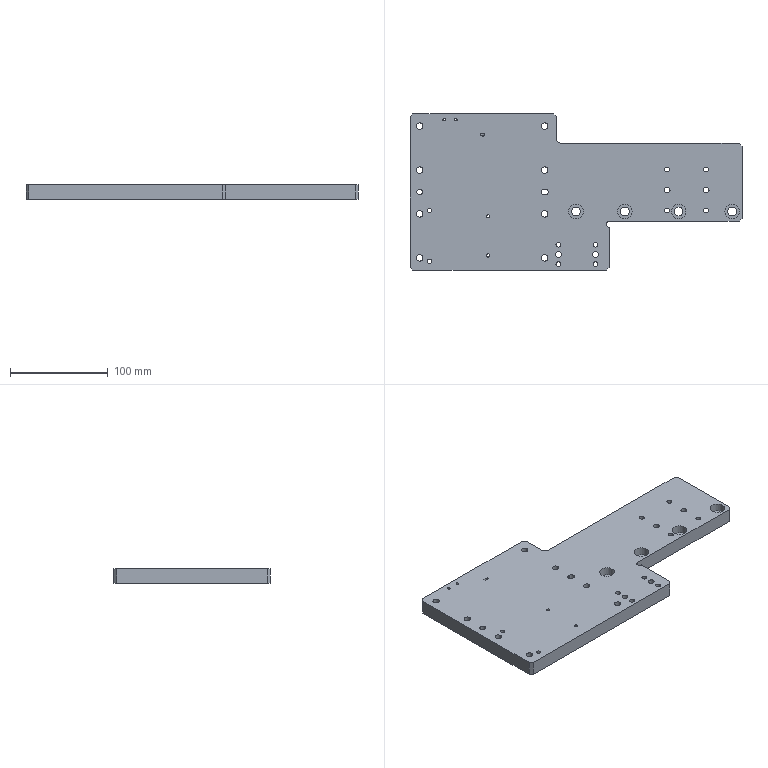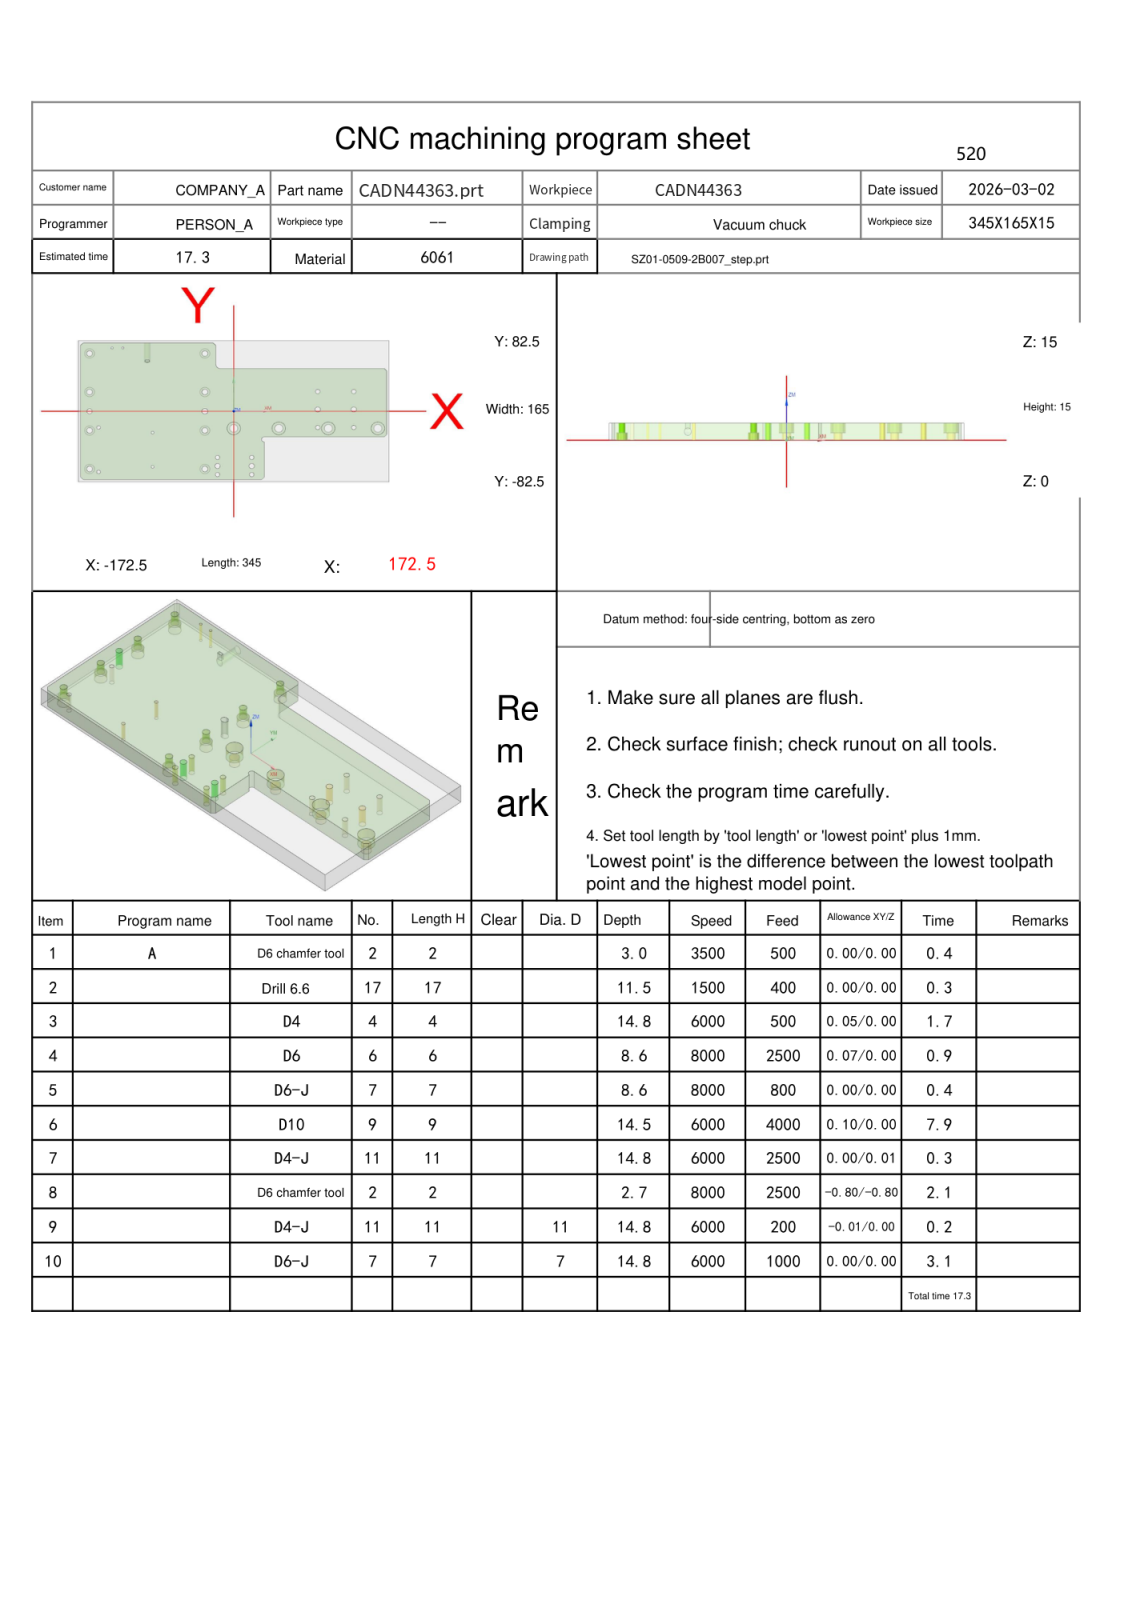NC program | NX | posted by the shop | part box 340 x 160 x 15 mm
Lines 978 to 1830 of 3961:
N6 T09 M06
(D10  D=10. R=0. H=09 ce=0.10 di=0.00)
G00 G90 G54 X-68. Y-85.1 M03 S6000
G43 H09 Z65.
M08
Z15.5
G01 X-167. Z15.451 F4000.
G02 X-170.606 Y-83.606 Z15.449 I0.0 J5.1
G01 X-173.606 Y-80.606 Z15.447
G02 X-175.1 Y-77. Z15.445 I3.606 J3.606
G01 Y77. Z15.37
G02 X-173.606 Y80.606 Z15.368 I5.1 J0.0
G01 X-170.606 Y83.606 Z15.366
G02 X-167. Y85.1 Z15.364 I3.606 J-3.606
G01 X-23. Z15.293
G02 X-19.394 Y83.606 Z15.291 I0.0 J-5.1
G01 X-16.394 Y80.606 Z15.289
G02 X-14.9 Y77. Z15.287 I-3.606 J-3.606
G01 Y55.1 Z15.276
X167. Z15.187
G02 X170.606 Y53.606 Z15.185 I0.0 J-5.1
G01 X173.606 Y50.606 Z15.183
G02 X175.1 Y47. Z15.181 I-3.606 J-3.606
G01 Y-27. Z15.144
G02 X173.606 Y-30.606 Z15.142 I-5.1 J0.0
G01 X170.606 Y-33.606 Z15.14
G02 X167. Y-35.1 Z15.138 I-3.606 J3.606
G01 X39.02 Z15.075
G02 X39.1 Y-36. Z15.075 I-5.02 J-.9
G01 Y-77. Z15.055
G02 X37.606 Y-80.606 Z15.053 I-5.1 J0.0
G01 X34.606 Y-83.606 Z15.051
G02 X31. Y-85.1 Z15.049 I-3.606 J3.606
G01 X-167. Z14.951
G02 X-170.606 Y-83.606 Z14.949 I0.0 J5.1
G01 X-173.606 Y-80.606 Z14.947
G02 X-175.1 Y-77. Z14.945 I3.606 J3.606
G01 Y77. Z14.87
G02 X-173.606 Y80.606 Z14.868 I5.1 J0.0
G01 X-170.606 Y83.606 Z14.866
G02 X-167. Y85.1 Z14.864 I3.606 J-3.606
G01 X-23. Z14.793
G02 X-19.394 Y83.606 Z14.791 I0.0 J-5.1
G01 X-16.394 Y80.606 Z14.789
G02 X-14.9 Y77. Z14.787 I-3.606 J-3.606
G01 Y55.1 Z14.776
X167. Z14.687
G02 X170.606 Y53.606 Z14.685 I0.0 J-5.1
G01 X173.606 Y50.606 Z14.683
G02 X175.1 Y47. Z14.681 I-3.606 J-3.606
G01 Y-27. Z14.644
G02 X173.606 Y-30.606 Z14.642 I-5.1 J0.0
G01 X170.606 Y-33.606 Z14.64
G02 X167. Y-35.1 Z14.638 I-3.606 J3.606
G01 X39.02 Z14.575
G02 X39.1 Y-36. Z14.575 I-5.02 J-.9
G01 Y-77. Z14.555
G02 X37.606 Y-80.606 Z14.553 I-5.1 J0.0
G01 X34.606 Y-83.606 Z14.551
G02 X31. Y-85.1 Z14.549 I-3.606 J3.606
G01 X-167. Z14.451
G02 X-170.606 Y-83.606 Z14.449 I0.0 J5.1
G01 X-173.606 Y-80.606 Z14.447
G02 X-175.1 Y-77. Z14.445 I3.606 J3.606
G01 Y77. Z14.37
G02 X-173.606 Y80.606 Z14.368 I5.1 J0.0
G01 X-170.606 Y83.606 Z14.366
G02 X-167. Y85.1 Z14.364 I3.606 J-3.606
G01 X-23. Z14.293
G02 X-19.394 Y83.606 Z14.291 I0.0 J-5.1
G01 X-16.394 Y80.606 Z14.289
G02 X-14.9 Y77. Z14.287 I-3.606 J-3.606
G01 Y55.1 Z14.276
X167. Z14.187
G02 X170.606 Y53.606 Z14.185 I0.0 J-5.1
G01 X173.606 Y50.606 Z14.183
G02 X175.1 Y47. Z14.181 I-3.606 J-3.606
G01 Y-27. Z14.144
G02 X173.606 Y-30.606 Z14.142 I-5.1 J0.0
G01 X170.606 Y-33.606 Z14.14
G02 X167. Y-35.1 Z14.138 I-3.606 J3.606
G01 X39.02 Z14.075
G02 X39.1 Y-36. Z14.075 I-5.02 J-.9
G01 Y-77. Z14.055
G02 X37.606 Y-80.606 Z14.053 I-5.1 J0.0
G01 X34.606 Y-83.606 Z14.051
G02 X31. Y-85.1 Z14.049 I-3.606 J3.606
G01 X-167. Z13.951
G02 X-170.606 Y-83.606 Z13.949 I0.0 J5.1
G01 X-173.606 Y-80.606 Z13.947
G02 X-175.1 Y-77. Z13.945 I3.606 J3.606
G01 Y77. Z13.87
G02 X-173.606 Y80.606 Z13.868 I5.1 J0.0
G01 X-170.606 Y83.606 Z13.866
G02 X-167. Y85.1 Z13.864 I3.606 J-3.606
G01 X-23. Z13.793
G02 X-19.394 Y83.606 Z13.791 I0.0 J-5.1
G01 X-16.394 Y80.606 Z13.789
G02 X-14.9 Y77. Z13.787 I-3.606 J-3.606
G01 Y55.1 Z13.776
X167. Z13.687
G02 X170.606 Y53.606 Z13.685 I0.0 J-5.1
G01 X173.606 Y50.606 Z13.683
G02 X175.1 Y47. Z13.681 I-3.606 J-3.606
G01 Y-27. Z13.644
G02 X173.606 Y-30.606 Z13.642 I-5.1 J0.0
G01 X170.606 Y-33.606 Z13.64
G02 X167. Y-35.1 Z13.638 I-3.606 J3.606
G01 X39.02 Z13.575
G02 X39.1 Y-36. Z13.575 I-5.02 J-.9
G01 Y-77. Z13.555
G02 X37.606 Y-80.606 Z13.553 I-5.1 J0.0
G01 X34.606 Y-83.606 Z13.551
G02 X31. Y-85.1 Z13.549 I-3.606 J3.606
G01 X-167. Z13.451
G02 X-170.606 Y-83.606 Z13.449 I0.0 J5.1
G01 X-173.606 Y-80.606 Z13.447
G02 X-175.1 Y-77. Z13.445 I3.606 J3.606
G01 Y77. Z13.37
G02 X-173.606 Y80.606 Z13.368 I5.1 J0.0
G01 X-170.606 Y83.606 Z13.366
G02 X-167. Y85.1 Z13.364 I3.606 J-3.606
G01 X-23. Z13.293
G02 X-19.394 Y83.606 Z13.291 I0.0 J-5.1
G01 X-16.394 Y80.606 Z13.289
G02 X-14.9 Y77. Z13.287 I-3.606 J-3.606
G01 Y55.1 Z13.276
X167. Z13.187
G02 X170.606 Y53.606 Z13.185 I0.0 J-5.1
G01 X173.606 Y50.606 Z13.183
G02 X175.1 Y47. Z13.181 I-3.606 J-3.606
G01 Y-27. Z13.144
G02 X173.606 Y-30.606 Z13.142 I-5.1 J0.0
G01 X170.606 Y-33.606 Z13.14
G02 X167. Y-35.1 Z13.138 I-3.606 J3.606
G01 X39.02 Z13.075
G02 X39.1 Y-36. Z13.075 I-5.02 J-.9
G01 Y-77. Z13.055
G02 X37.606 Y-80.606 Z13.053 I-5.1 J0.0
G01 X34.606 Y-83.606 Z13.051
G02 X31. Y-85.1 Z13.049 I-3.606 J3.606
G01 X-167. Z12.951
G02 X-170.606 Y-83.606 Z12.949 I0.0 J5.1
G01 X-173.606 Y-80.606 Z12.947
G02 X-175.1 Y-77. Z12.945 I3.606 J3.606
G01 Y77. Z12.87
G02 X-173.606 Y80.606 Z12.868 I5.1 J0.0
G01 X-170.606 Y83.606 Z12.866
G02 X-167. Y85.1 Z12.864 I3.606 J-3.606
G01 X-23. Z12.793
G02 X-19.394 Y83.606 Z12.791 I0.0 J-5.1
G01 X-16.394 Y80.606 Z12.789
G02 X-14.9 Y77. Z12.787 I-3.606 J-3.606
G01 Y55.1 Z12.776
X167. Z12.687
G02 X170.606 Y53.606 Z12.685 I0.0 J-5.1
G01 X173.606 Y50.606 Z12.683
G02 X175.1 Y47. Z12.681 I-3.606 J-3.606
G01 Y-27. Z12.644
G02 X173.606 Y-30.606 Z12.642 I-5.1 J0.0
G01 X170.606 Y-33.606 Z12.64
G02 X167. Y-35.1 Z12.638 I-3.606 J3.606
G01 X39.02 Z12.575
G02 X39.1 Y-36. Z12.575 I-5.02 J-.9
G01 Y-77. Z12.555
G02 X37.606 Y-80.606 Z12.553 I-5.1 J0.0
G01 X34.606 Y-83.606 Z12.551
G02 X31. Y-85.1 Z12.549 I-3.606 J3.606
G01 X-167. Z12.451
G02 X-170.606 Y-83.606 Z12.449 I0.0 J5.1
G01 X-173.606 Y-80.606 Z12.447
G02 X-175.1 Y-77. Z12.445 I3.606 J3.606
G01 Y77. Z12.37
G02 X-173.606 Y80.606 Z12.368 I5.1 J0.0
G01 X-170.606 Y83.606 Z12.366
G02 X-167. Y85.1 Z12.364 I3.606 J-3.606
G01 X-23. Z12.293
G02 X-19.394 Y83.606 Z12.291 I0.0 J-5.1
G01 X-16.394 Y80.606 Z12.289
G02 X-14.9 Y77. Z12.287 I-3.606 J-3.606
G01 Y55.1 Z12.276
X167. Z12.187
G02 X170.606 Y53.606 Z12.185 I0.0 J-5.1
G01 X173.606 Y50.606 Z12.183
G02 X175.1 Y47. Z12.181 I-3.606 J-3.606
G01 Y-27. Z12.144
G02 X173.606 Y-30.606 Z12.142 I-5.1 J0.0
G01 X170.606 Y-33.606 Z12.14
G02 X167. Y-35.1 Z12.138 I-3.606 J3.606
G01 X39.02 Z12.075
G02 X39.1 Y-36. Z12.075 I-5.02 J-.9
G01 Y-77. Z12.055
G02 X37.606 Y-80.606 Z12.053 I-5.1 J0.0
G01 X34.606 Y-83.606 Z12.051
G02 X31. Y-85.1 Z12.049 I-3.606 J3.606
G01 X-167. Z11.951
G02 X-170.606 Y-83.606 Z11.949 I0.0 J5.1
G01 X-173.606 Y-80.606 Z11.947
G02 X-175.1 Y-77. Z11.945 I3.606 J3.606
G01 Y77. Z11.87
G02 X-173.606 Y80.606 Z11.868 I5.1 J0.0
G01 X-170.606 Y83.606 Z11.866
G02 X-167. Y85.1 Z11.864 I3.606 J-3.606
G01 X-23. Z11.793
G02 X-19.394 Y83.606 Z11.791 I0.0 J-5.1
G01 X-16.394 Y80.606 Z11.789
G02 X-14.9 Y77. Z11.787 I-3.606 J-3.606
G01 Y55.1 Z11.776
X167. Z11.687
G02 X170.606 Y53.606 Z11.685 I0.0 J-5.1
G01 X173.606 Y50.606 Z11.683
G02 X175.1 Y47. Z11.681 I-3.606 J-3.606
G01 Y-27. Z11.644
G02 X173.606 Y-30.606 Z11.642 I-5.1 J0.0
G01 X170.606 Y-33.606 Z11.64
G02 X167. Y-35.1 Z11.638 I-3.606 J3.606
G01 X39.02 Z11.575
G02 X39.1 Y-36. Z11.575 I-5.02 J-.9
G01 Y-77. Z11.555
G02 X37.606 Y-80.606 Z11.553 I-5.1 J0.0
G01 X34.606 Y-83.606 Z11.551
G02 X31. Y-85.1 Z11.549 I-3.606 J3.606
G01 X-167. Z11.451
G02 X-170.606 Y-83.606 Z11.449 I0.0 J5.1
G01 X-173.606 Y-80.606 Z11.447
G02 X-175.1 Y-77. Z11.445 I3.606 J3.606
G01 Y77. Z11.37
G02 X-173.606 Y80.606 Z11.368 I5.1 J0.0
G01 X-170.606 Y83.606 Z11.366
G02 X-167. Y85.1 Z11.364 I3.606 J-3.606
G01 X-23. Z11.293
G02 X-19.394 Y83.606 Z11.291 I0.0 J-5.1
G01 X-16.394 Y80.606 Z11.289
G02 X-14.9 Y77. Z11.287 I-3.606 J-3.606
G01 Y55.1 Z11.276
X167. Z11.187
G02 X170.606 Y53.606 Z11.185 I0.0 J-5.1
G01 X173.606 Y50.606 Z11.183
G02 X175.1 Y47. Z11.181 I-3.606 J-3.606
G01 Y-27. Z11.144
G02 X173.606 Y-30.606 Z11.142 I-5.1 J0.0
G01 X170.606 Y-33.606 Z11.14
G02 X167. Y-35.1 Z11.138 I-3.606 J3.606
G01 X39.02 Z11.075
G02 X39.1 Y-36. Z11.075 I-5.02 J-.9
G01 Y-77. Z11.055
G02 X37.606 Y-80.606 Z11.053 I-5.1 J0.0
G01 X34.606 Y-83.606 Z11.051
G02 X31. Y-85.1 Z11.049 I-3.606 J3.606
G01 X-167. Z10.951
G02 X-170.606 Y-83.606 Z10.949 I0.0 J5.1
G01 X-173.606 Y-80.606 Z10.947
G02 X-175.1 Y-77. Z10.945 I3.606 J3.606
G01 Y77. Z10.87
G02 X-173.606 Y80.606 Z10.868 I5.1 J0.0
G01 X-170.606 Y83.606 Z10.866
G02 X-167. Y85.1 Z10.864 I3.606 J-3.606
G01 X-23. Z10.793
G02 X-19.394 Y83.606 Z10.791 I0.0 J-5.1
G01 X-16.394 Y80.606 Z10.789
G02 X-14.9 Y77. Z10.787 I-3.606 J-3.606
G01 Y55.1 Z10.776
X167. Z10.687
G02 X170.606 Y53.606 Z10.685 I0.0 J-5.1
G01 X173.606 Y50.606 Z10.683
G02 X175.1 Y47. Z10.681 I-3.606 J-3.606
G01 Y-27. Z10.644
G02 X173.606 Y-30.606 Z10.642 I-5.1 J0.0
G01 X170.606 Y-33.606 Z10.64
G02 X167. Y-35.1 Z10.638 I-3.606 J3.606
G01 X39.02 Z10.575
G02 X39.1 Y-36. Z10.575 I-5.02 J-.9
G01 Y-77. Z10.555
G02 X37.606 Y-80.606 Z10.553 I-5.1 J0.0
G01 X34.606 Y-83.606 Z10.551
G02 X31. Y-85.1 Z10.549 I-3.606 J3.606
G01 X-167. Z10.451
G02 X-170.606 Y-83.606 Z10.449 I0.0 J5.1
G01 X-173.606 Y-80.606 Z10.447
G02 X-175.1 Y-77. Z10.445 I3.606 J3.606
G01 Y77. Z10.37
G02 X-173.606 Y80.606 Z10.368 I5.1 J0.0
G01 X-170.606 Y83.606 Z10.366
G02 X-167. Y85.1 Z10.364 I3.606 J-3.606
G01 X-23. Z10.293
G02 X-19.394 Y83.606 Z10.291 I0.0 J-5.1
G01 X-16.394 Y80.606 Z10.289
G02 X-14.9 Y77. Z10.287 I-3.606 J-3.606
G01 Y55.1 Z10.276
X167. Z10.187
G02 X170.606 Y53.606 Z10.185 I0.0 J-5.1
G01 X173.606 Y50.606 Z10.183
G02 X175.1 Y47. Z10.181 I-3.606 J-3.606
G01 Y-27. Z10.144
G02 X173.606 Y-30.606 Z10.142 I-5.1 J0.0
G01 X170.606 Y-33.606 Z10.14
G02 X167. Y-35.1 Z10.138 I-3.606 J3.606
G01 X39.02 Z10.075
G02 X39.1 Y-36. Z10.075 I-5.02 J-.9
G01 Y-77. Z10.055
G02 X37.606 Y-80.606 Z10.053 I-5.1 J0.0
G01 X34.606 Y-83.606 Z10.051
G02 X31. Y-85.1 Z10.049 I-3.606 J3.606
G01 X-167. Z9.951
G02 X-170.606 Y-83.606 Z9.949 I0.0 J5.1
G01 X-173.606 Y-80.606 Z9.947
G02 X-175.1 Y-77. Z9.945 I3.606 J3.606
G01 Y77. Z9.87
G02 X-173.606 Y80.606 Z9.868 I5.1 J0.0
G01 X-170.606 Y83.606 Z9.866
G02 X-167. Y85.1 Z9.864 I3.606 J-3.606
G01 X-23. Z9.793
G02 X-19.394 Y83.606 Z9.791 I0.0 J-5.1
G01 X-16.394 Y80.606 Z9.789
G02 X-14.9 Y77. Z9.787 I-3.606 J-3.606
G01 Y55.1 Z9.776
X167. Z9.687
G02 X170.606 Y53.606 Z9.685 I0.0 J-5.1
G01 X173.606 Y50.606 Z9.683
G02 X175.1 Y47. Z9.681 I-3.606 J-3.606
G01 Y-27. Z9.644
G02 X173.606 Y-30.606 Z9.642 I-5.1 J0.0
G01 X170.606 Y-33.606 Z9.64
G02 X167. Y-35.1 Z9.638 I-3.606 J3.606
G01 X39.02 Z9.575
G02 X39.1 Y-36. Z9.575 I-5.02 J-.9
G01 Y-77. Z9.555
G02 X37.606 Y-80.606 Z9.553 I-5.1 J0.0
G01 X34.606 Y-83.606 Z9.551
G02 X31. Y-85.1 Z9.549 I-3.606 J3.606
G01 X-167. Z9.451
G02 X-170.606 Y-83.606 Z9.449 I0.0 J5.1
G01 X-173.606 Y-80.606 Z9.447
G02 X-175.1 Y-77. Z9.445 I3.606 J3.606
G01 Y77. Z9.37
G02 X-173.606 Y80.606 Z9.368 I5.1 J0.0
G01 X-170.606 Y83.606 Z9.366
G02 X-167. Y85.1 Z9.364 I3.606 J-3.606
G01 X-23. Z9.293
G02 X-19.394 Y83.606 Z9.291 I0.0 J-5.1
G01 X-16.394 Y80.606 Z9.289
G02 X-14.9 Y77. Z9.287 I-3.606 J-3.606
G01 Y55.1 Z9.276
X167. Z9.187
G02 X170.606 Y53.606 Z9.185 I0.0 J-5.1
G01 X173.606 Y50.606 Z9.183
G02 X175.1 Y47. Z9.181 I-3.606 J-3.606
G01 Y-27. Z9.144
G02 X173.606 Y-30.606 Z9.142 I-5.1 J0.0
G01 X170.606 Y-33.606 Z9.14
G02 X167. Y-35.1 Z9.138 I-3.606 J3.606
G01 X39.02 Z9.075
G02 X39.1 Y-36. Z9.075 I-5.02 J-.9
G01 Y-77. Z9.055
G02 X37.606 Y-80.606 Z9.053 I-5.1 J0.0
G01 X34.606 Y-83.606 Z9.051
G02 X31. Y-85.1 Z9.049 I-3.606 J3.606
G01 X-167. Z8.951
G02 X-170.606 Y-83.606 Z8.949 I0.0 J5.1
G01 X-173.606 Y-80.606 Z8.947
G02 X-175.1 Y-77. Z8.945 I3.606 J3.606
G01 Y77. Z8.87
G02 X-173.606 Y80.606 Z8.868 I5.1 J0.0
G01 X-170.606 Y83.606 Z8.866
G02 X-167. Y85.1 Z8.864 I3.606 J-3.606
G01 X-23. Z8.793
G02 X-19.394 Y83.606 Z8.791 I0.0 J-5.1
G01 X-16.394 Y80.606 Z8.789
G02 X-14.9 Y77. Z8.787 I-3.606 J-3.606
G01 Y55.1 Z8.776
X167. Z8.687
G02 X170.606 Y53.606 Z8.685 I0.0 J-5.1
G01 X173.606 Y50.606 Z8.683
G02 X175.1 Y47. Z8.681 I-3.606 J-3.606
G01 Y-27. Z8.644
G02 X173.606 Y-30.606 Z8.642 I-5.1 J0.0
G01 X170.606 Y-33.606 Z8.64
G02 X167. Y-35.1 Z8.638 I-3.606 J3.606
G01 X39.02 Z8.575
G02 X39.1 Y-36. Z8.575 I-5.02 J-.9
G01 Y-77. Z8.555
G02 X37.606 Y-80.606 Z8.553 I-5.1 J0.0
G01 X34.606 Y-83.606 Z8.551
G02 X31. Y-85.1 Z8.549 I-3.606 J3.606
G01 X-167. Z8.451
G02 X-170.606 Y-83.606 Z8.449 I0.0 J5.1
G01 X-173.606 Y-80.606 Z8.447
G02 X-175.1 Y-77. Z8.445 I3.606 J3.606
G01 Y77. Z8.37
G02 X-173.606 Y80.606 Z8.368 I5.1 J0.0
G01 X-170.606 Y83.606 Z8.366
G02 X-167. Y85.1 Z8.364 I3.606 J-3.606
G01 X-23. Z8.293
G02 X-19.394 Y83.606 Z8.291 I0.0 J-5.1
G01 X-16.394 Y80.606 Z8.289
G02 X-14.9 Y77. Z8.287 I-3.606 J-3.606
G01 Y55.1 Z8.276
X167. Z8.187
G02 X170.606 Y53.606 Z8.185 I0.0 J-5.1
G01 X173.606 Y50.606 Z8.183
G02 X175.1 Y47. Z8.181 I-3.606 J-3.606
G01 Y-27. Z8.144
G02 X173.606 Y-30.606 Z8.142 I-5.1 J0.0
G01 X170.606 Y-33.606 Z8.14
G02 X167. Y-35.1 Z8.138 I-3.606 J3.606
G01 X39.02 Z8.075
G02 X39.1 Y-36. Z8.075 I-5.02 J-.9
G01 Y-77. Z8.055
G02 X37.606 Y-80.606 Z8.053 I-5.1 J0.0
G01 X34.606 Y-83.606 Z8.051
G02 X31. Y-85.1 Z8.049 I-3.606 J3.606
G01 X-167. Z7.951
G02 X-170.606 Y-83.606 Z7.949 I0.0 J5.1
G01 X-173.606 Y-80.606 Z7.947
G02 X-175.1 Y-77. Z7.945 I3.606 J3.606
G01 Y77. Z7.87
G02 X-173.606 Y80.606 Z7.868 I5.1 J0.0
G01 X-170.606 Y83.606 Z7.866
G02 X-167. Y85.1 Z7.864 I3.606 J-3.606
G01 X-23. Z7.793
G02 X-19.394 Y83.606 Z7.791 I0.0 J-5.1
G01 X-16.394 Y80.606 Z7.789
G02 X-14.9 Y77. Z7.787 I-3.606 J-3.606
G01 Y55.1 Z7.776
X167. Z7.687
G02 X170.606 Y53.606 Z7.685 I0.0 J-5.1
G01 X173.606 Y50.606 Z7.683
G02 X175.1 Y47. Z7.681 I-3.606 J-3.606
G01 Y-27. Z7.644
G02 X173.606 Y-30.606 Z7.642 I-5.1 J0.0
G01 X170.606 Y-33.606 Z7.64
G02 X167. Y-35.1 Z7.638 I-3.606 J3.606
G01 X39.02 Z7.575
G02 X39.1 Y-36. Z7.575 I-5.02 J-.9
G01 Y-77. Z7.555
G02 X37.606 Y-80.606 Z7.553 I-5.1 J0.0
G01 X34.606 Y-83.606 Z7.551
G02 X31. Y-85.1 Z7.549 I-3.606 J3.606
G01 X-167. Z7.451
G02 X-170.606 Y-83.606 Z7.449 I0.0 J5.1
G01 X-173.606 Y-80.606 Z7.447
G02 X-175.1 Y-77. Z7.445 I3.606 J3.606
G01 Y77. Z7.37
G02 X-173.606 Y80.606 Z7.368 I5.1 J0.0
G01 X-170.606 Y83.606 Z7.366
G02 X-167. Y85.1 Z7.364 I3.606 J-3.606
G01 X-23. Z7.293
G02 X-19.394 Y83.606 Z7.291 I0.0 J-5.1
G01 X-16.394 Y80.606 Z7.289
G02 X-14.9 Y77. Z7.287 I-3.606 J-3.606
G01 Y55.1 Z7.276
X167. Z7.187
G02 X170.606 Y53.606 Z7.185 I0.0 J-5.1
G01 X173.606 Y50.606 Z7.183
G02 X175.1 Y47. Z7.181 I-3.606 J-3.606
G01 Y-27. Z7.144
G02 X173.606 Y-30.606 Z7.142 I-5.1 J0.0
G01 X170.606 Y-33.606 Z7.14
G02 X167. Y-35.1 Z7.138 I-3.606 J3.606
G01 X39.02 Z7.075
G02 X39.1 Y-36. Z7.075 I-5.02 J-.9
G01 Y-77. Z7.055
G02 X37.606 Y-80.606 Z7.053 I-5.1 J0.0
G01 X34.606 Y-83.606 Z7.051
G02 X31. Y-85.1 Z7.049 I-3.606 J3.606
G01 X-167. Z6.951
G02 X-170.606 Y-83.606 Z6.949 I0.0 J5.1
G01 X-173.606 Y-80.606 Z6.947
G02 X-175.1 Y-77. Z6.945 I3.606 J3.606
G01 Y77. Z6.87
G02 X-173.606 Y80.606 Z6.868 I5.1 J0.0
G01 X-170.606 Y83.606 Z6.866
G02 X-167. Y85.1 Z6.864 I3.606 J-3.606
G01 X-23. Z6.793
G02 X-19.394 Y83.606 Z6.791 I0.0 J-5.1
G01 X-16.394 Y80.606 Z6.789
G02 X-14.9 Y77. Z6.787 I-3.606 J-3.606
G01 Y55.1 Z6.776
X167. Z6.687
G02 X170.606 Y53.606 Z6.685 I0.0 J-5.1
G01 X173.606 Y50.606 Z6.683
G02 X175.1 Y47. Z6.681 I-3.606 J-3.606
G01 Y-27. Z6.644
G02 X173.606 Y-30.606 Z6.642 I-5.1 J0.0
G01 X170.606 Y-33.606 Z6.64
G02 X167. Y-35.1 Z6.638 I-3.606 J3.606
G01 X39.02 Z6.575
G02 X39.1 Y-36. Z6.575 I-5.02 J-.9
G01 Y-77. Z6.555
G02 X37.606 Y-80.606 Z6.553 I-5.1 J0.0
G01 X34.606 Y-83.606 Z6.551
G02 X31. Y-85.1 Z6.549 I-3.606 J3.606
G01 X-167. Z6.451
G02 X-170.606 Y-83.606 Z6.449 I0.0 J5.1
G01 X-173.606 Y-80.606 Z6.447
G02 X-175.1 Y-77. Z6.445 I3.606 J3.606
G01 Y77. Z6.37
G02 X-173.606 Y80.606 Z6.368 I5.1 J0.0
G01 X-170.606 Y83.606 Z6.366
G02 X-167. Y85.1 Z6.364 I3.606 J-3.606
G01 X-23. Z6.293
G02 X-19.394 Y83.606 Z6.291 I0.0 J-5.1
G01 X-16.394 Y80.606 Z6.289
G02 X-14.9 Y77. Z6.287 I-3.606 J-3.606
G01 Y55.1 Z6.276
X167. Z6.187
G02 X170.606 Y53.606 Z6.185 I0.0 J-5.1
G01 X173.606 Y50.606 Z6.183
G02 X175.1 Y47. Z6.181 I-3.606 J-3.606
G01 Y-27. Z6.144
G02 X173.606 Y-30.606 Z6.142 I-5.1 J0.0
G01 X170.606 Y-33.606 Z6.14
G02 X167. Y-35.1 Z6.138 I-3.606 J3.606
G01 X39.02 Z6.075
G02 X39.1 Y-36. Z6.075 I-5.02 J-.9
G01 Y-77. Z6.055
G02 X37.606 Y-80.606 Z6.053 I-5.1 J0.0
G01 X34.606 Y-83.606 Z6.051
G02 X31. Y-85.1 Z6.049 I-3.606 J3.606
G01 X-167. Z5.951
G02 X-170.606 Y-83.606 Z5.949 I0.0 J5.1
G01 X-173.606 Y-80.606 Z5.947
G02 X-175.1 Y-77. Z5.945 I3.606 J3.606
G01 Y77. Z5.87
G02 X-173.606 Y80.606 Z5.868 I5.1 J0.0
G01 X-170.606 Y83.606 Z5.866
G02 X-167. Y85.1 Z5.864 I3.606 J-3.606
G01 X-23. Z5.793
G02 X-19.394 Y83.606 Z5.791 I0.0 J-5.1
G01 X-16.394 Y80.606 Z5.789
G02 X-14.9 Y77. Z5.787 I-3.606 J-3.606
G01 Y55.1 Z5.776
X167. Z5.687
G02 X170.606 Y53.606 Z5.685 I0.0 J-5.1
G01 X173.606 Y50.606 Z5.683
G02 X175.1 Y47. Z5.681 I-3.606 J-3.606
G01 Y-27. Z5.644
G02 X173.606 Y-30.606 Z5.642 I-5.1 J0.0
G01 X170.606 Y-33.606 Z5.64
G02 X167. Y-35.1 Z5.638 I-3.606 J3.606
G01 X39.02 Z5.575
G02 X39.1 Y-36. Z5.575 I-5.02 J-.9
G01 Y-77. Z5.555
G02 X37.606 Y-80.606 Z5.553 I-5.1 J0.0
G01 X34.606 Y-83.606 Z5.551
G02 X31. Y-85.1 Z5.549 I-3.606 J3.606
G01 X-167. Z5.451
G02 X-170.606 Y-83.606 Z5.449 I0.0 J5.1
G01 X-173.606 Y-80.606 Z5.447
G02 X-175.1 Y-77. Z5.445 I3.606 J3.606
G01 Y77. Z5.37
G02 X-173.606 Y80.606 Z5.368 I5.1 J0.0
G01 X-170.606 Y83.606 Z5.366
G02 X-167. Y85.1 Z5.364 I3.606 J-3.606
G01 X-23. Z5.293
G02 X-19.394 Y83.606 Z5.291 I0.0 J-5.1
G01 X-16.394 Y80.606 Z5.289
G02 X-14.9 Y77. Z5.287 I-3.606 J-3.606
G01 Y55.1 Z5.276
X167. Z5.187
G02 X170.606 Y53.606 Z5.185 I0.0 J-5.1
G01 X173.606 Y50.606 Z5.183
G02 X175.1 Y47. Z5.181 I-3.606 J-3.606
G01 Y-27. Z5.144
G02 X173.606 Y-30.606 Z5.142 I-5.1 J0.0
G01 X170.606 Y-33.606 Z5.14
G02 X167. Y-35.1 Z5.138 I-3.606 J3.606
G01 X39.02 Z5.075
G02 X39.1 Y-36. Z5.075 I-5.02 J-.9
G01 Y-77. Z5.055
G02 X37.606 Y-80.606 Z5.053 I-5.1 J0.0
G01 X34.606 Y-83.606 Z5.051
G02 X31. Y-85.1 Z5.049 I-3.606 J3.606
G01 X-167. Z4.951
G02 X-170.606 Y-83.606 Z4.949 I0.0 J5.1
G01 X-173.606 Y-80.606 Z4.947
G02 X-175.1 Y-77. Z4.945 I3.606 J3.606
G01 Y77. Z4.87
G02 X-173.606 Y80.606 Z4.868 I5.1 J0.0
G01 X-170.606 Y83.606 Z4.866
G02 X-167. Y85.1 Z4.864 I3.606 J-3.606
G01 X-23. Z4.793
G02 X-19.394 Y83.606 Z4.791 I0.0 J-5.1
G01 X-16.394 Y80.606 Z4.789
G02 X-14.9 Y77. Z4.787 I-3.606 J-3.606
G01 Y55.1 Z4.776
X167. Z4.687
G02 X170.606 Y53.606 Z4.685 I0.0 J-5.1
G01 X173.606 Y50.606 Z4.683
G02 X175.1 Y47. Z4.681 I-3.606 J-3.606
G01 Y-27. Z4.644
G02 X173.606 Y-30.606 Z4.642 I-5.1 J0.0
G01 X170.606 Y-33.606 Z4.64
G02 X167. Y-35.1 Z4.638 I-3.606 J3.606
G01 X39.02 Z4.575
G02 X39.1 Y-36. Z4.575 I-5.02 J-.9
G01 Y-77. Z4.555
G02 X37.606 Y-80.606 Z4.553 I-5.1 J0.0
G01 X34.606 Y-83.606 Z4.551
G02 X31. Y-85.1 Z4.549 I-3.606 J3.606
G01 X-167. Z4.451
G02 X-170.606 Y-83.606 Z4.449 I0.0 J5.1
G01 X-173.606 Y-80.606 Z4.447
G02 X-175.1 Y-77. Z4.445 I3.606 J3.606
G01 Y77. Z4.37
G02 X-173.606 Y80.606 Z4.368 I5.1 J0.0
G01 X-170.606 Y83.606 Z4.366
G02 X-167. Y85.1 Z4.364 I3.606 J-3.606
G01 X-23. Z4.293
G02 X-19.394 Y83.606 Z4.291 I0.0 J-5.1
G01 X-16.394 Y80.606 Z4.289
G02 X-14.9 Y77. Z4.287 I-3.606 J-3.606
G01 Y55.1 Z4.276
X167. Z4.187
G02 X170.606 Y53.606 Z4.185 I0.0 J-5.1
G01 X173.606 Y50.606 Z4.183
G02 X175.1 Y47. Z4.181 I-3.606 J-3.606
G01 Y-27. Z4.144
G02 X173.606 Y-30.606 Z4.142 I-5.1 J0.0
G01 X170.606 Y-33.606 Z4.14
G02 X167. Y-35.1 Z4.138 I-3.606 J3.606
G01 X39.02 Z4.075
G02 X39.1 Y-36. Z4.075 I-5.02 J-.9
G01 Y-77. Z4.055
G02 X37.606 Y-80.606 Z4.053 I-5.1 J0.0
G01 X34.606 Y-83.606 Z4.051
G02 X31. Y-85.1 Z4.049 I-3.606 J3.606
G01 X-167. Z3.951
G02 X-170.606 Y-83.606 Z3.949 I0.0 J5.1
G01 X-173.606 Y-80.606 Z3.947
G02 X-175.1 Y-77. Z3.945 I3.606 J3.606
G01 Y77. Z3.87
G02 X-173.606 Y80.606 Z3.868 I5.1 J0.0
G01 X-170.606 Y83.606 Z3.866
G02 X-167. Y85.1 Z3.864 I3.606 J-3.606
G01 X-23. Z3.793
G02 X-19.394 Y83.606 Z3.791 I0.0 J-5.1
G01 X-16.394 Y80.606 Z3.789
G02 X-14.9 Y77. Z3.787 I-3.606 J-3.606
G01 Y55.1 Z3.776
X167. Z3.687
G02 X170.606 Y53.606 Z3.685 I0.0 J-5.1
G01 X173.606 Y50.606 Z3.683
G02 X175.1 Y47. Z3.681 I-3.606 J-3.606
G01 Y-27. Z3.644
G02 X173.606 Y-30.606 Z3.642 I-5.1 J0.0
G01 X170.606 Y-33.606 Z3.64
G02 X167. Y-35.1 Z3.638 I-3.606 J3.606
G01 X39.02 Z3.575
G02 X39.1 Y-36. Z3.575 I-5.02 J-.9
G01 Y-77. Z3.555
G02 X37.606 Y-80.606 Z3.553 I-5.1 J0.0
G01 X34.606 Y-83.606 Z3.551
G02 X31. Y-85.1 Z3.549 I-3.606 J3.606
G01 X-167. Z3.451
G02 X-170.606 Y-83.606 Z3.449 I0.0 J5.1
G01 X-173.606 Y-80.606 Z3.447
G02 X-175.1 Y-77. Z3.445 I3.606 J3.606
G01 Y77. Z3.37
G02 X-173.606 Y80.606 Z3.368 I5.1 J0.0
G01 X-170.606 Y83.606 Z3.366
G02 X-167. Y85.1 Z3.364 I3.606 J-3.606
G01 X-23. Z3.293
G02 X-19.394 Y83.606 Z3.291 I0.0 J-5.1
G01 X-16.394 Y80.606 Z3.289
G02 X-14.9 Y77. Z3.287 I-3.606 J-3.606
G01 Y55.1 Z3.276
X167. Z3.187
G02 X170.606 Y53.606 Z3.185 I0.0 J-5.1
G01 X173.606 Y50.606 Z3.183
G02 X175.1 Y47. Z3.181 I-3.606 J-3.606
G01 Y-27. Z3.144
G02 X173.606 Y-30.606 Z3.142 I-5.1 J0.0
G01 X170.606 Y-33.606 Z3.14
G02 X167. Y-35.1 Z3.138 I-3.606 J3.606
G01 X39.02 Z3.075
G02 X39.1 Y-36. Z3.075 I-5.02 J-.9
G01 Y-77. Z3.055
G02 X37.606 Y-80.606 Z3.053 I-5.1 J0.0
G01 X34.606 Y-83.606 Z3.051
G02 X31. Y-85.1 Z3.049 I-3.606 J3.606
G01 X-167. Z2.951
G02 X-170.606 Y-83.606 Z2.949 I0.0 J5.1
G01 X-173.606 Y-80.606 Z2.947
G02 X-175.1 Y-77. Z2.945 I3.606 J3.606
G01 Y77. Z2.87
G02 X-173.606 Y80.606 Z2.868 I5.1 J0.0
G01 X-170.606 Y83.606 Z2.866
G02 X-167. Y85.1 Z2.864 I3.606 J-3.606
G01 X-23. Z2.793
G02 X-19.394 Y83.606 Z2.791 I0.0 J-5.1
G01 X-16.394 Y80.606 Z2.789
G02 X-14.9 Y77. Z2.787 I-3.606 J-3.606
G01 Y55.1 Z2.776
X167. Z2.687
G02 X170.606 Y53.606 Z2.685 I0.0 J-5.1
G01 X173.606 Y50.606 Z2.683
G02 X175.1 Y47. Z2.681 I-3.606 J-3.606
G01 Y-27. Z2.644
G02 X173.606 Y-30.606 Z2.642 I-5.1 J0.0
G01 X170.606 Y-33.606 Z2.64
G02 X167. Y-35.1 Z2.638 I-3.606 J3.606
G01 X39.02 Z2.575
G02 X39.1 Y-36. Z2.575 I-5.02 J-.9
G01 Y-77. Z2.555
G02 X37.606 Y-80.606 Z2.553 I-5.1 J0.0
G01 X34.606 Y-83.606 Z2.551
G02 X31. Y-85.1 Z2.549 I-3.606 J3.606
G01 X-167. Z2.451
G02 X-170.606 Y-83.606 Z2.449 I0.0 J5.1
G01 X-173.606 Y-80.606 Z2.447
G02 X-175.1 Y-77. Z2.445 I3.606 J3.606
G01 Y77. Z2.37
G02 X-173.606 Y80.606 Z2.368 I5.1 J0.0
G01 X-170.606 Y83.606 Z2.366
G02 X-167. Y85.1 Z2.364 I3.606 J-3.606
G01 X-23. Z2.293
G02 X-19.394 Y83.606 Z2.291 I0.0 J-5.1
G01 X-16.394 Y80.606 Z2.289
G02 X-14.9 Y77. Z2.287 I-3.606 J-3.606
G01 Y55.1 Z2.276
X167. Z2.187
G02 X170.606 Y53.606 Z2.185 I0.0 J-5.1
G01 X173.606 Y50.606 Z2.183
G02 X175.1 Y47. Z2.181 I-3.606 J-3.606
G01 Y-27. Z2.144
G02 X173.606 Y-30.606 Z2.142 I-5.1 J0.0
G01 X170.606 Y-33.606 Z2.14
G02 X167. Y-35.1 Z2.138 I-3.606 J3.606
G01 X39.02 Z2.075
G02 X39.1 Y-36. Z2.075 I-5.02 J-.9
G01 Y-77. Z2.055
G02 X37.606 Y-80.606 Z2.053 I-5.1 J0.0
G01 X34.606 Y-83.606 Z2.051
G02 X31. Y-85.1 Z2.049 I-3.606 J3.606
G01 X-167. Z1.951
G02 X-170.606 Y-83.606 Z1.949 I0.0 J5.1
G01 X-173.606 Y-80.606 Z1.947
G02 X-175.1 Y-77. Z1.945 I3.606 J3.606
G01 Y77. Z1.87
G02 X-173.606 Y80.606 Z1.868 I5.1 J0.0
G01 X-170.606 Y83.606 Z1.866
G02 X-167. Y85.1 Z1.864 I3.606 J-3.606
G01 X-23. Z1.793
G02 X-19.394 Y83.606 Z1.791 I0.0 J-5.1
G01 X-16.394 Y80.606 Z1.789
G02 X-14.9 Y77. Z1.787 I-3.606 J-3.606
G01 Y55.1 Z1.776
X167. Z1.687
G02 X170.606 Y53.606 Z1.685 I0.0 J-5.1
G01 X173.606 Y50.606 Z1.683
G02 X175.1 Y47. Z1.681 I-3.606 J-3.606
G01 Y-27. Z1.644
G02 X173.606 Y-30.606 Z1.642 I-5.1 J0.0
G01 X170.606 Y-33.606 Z1.64
G02 X167. Y-35.1 Z1.638 I-3.606 J3.606
G01 X39.02 Z1.575
G02 X39.1 Y-36. Z1.575 I-5.02 J-.9
G01 Y-77. Z1.555
G02 X37.606 Y-80.606 Z1.553 I-5.1 J0.0
G01 X34.606 Y-83.606 Z1.551
G02 X31. Y-85.1 Z1.549 I-3.606 J3.606
G01 X-167. Z1.451
G02 X-170.606 Y-83.606 Z1.449 I0.0 J5.1
G01 X-173.606 Y-80.606 Z1.447
G02 X-175.1 Y-77. Z1.445 I3.606 J3.606
G01 Y77. Z1.37
G02 X-173.606 Y80.606 Z1.368 I5.1 J0.0
G01 X-170.606 Y83.606 Z1.366
G02 X-167. Y85.1 Z1.364 I3.606 J-3.606
G01 X-23. Z1.293
G02 X-19.394 Y83.606 Z1.291 I0.0 J-5.1
G01 X-16.394 Y80.606 Z1.289
G02 X-14.9 Y77. Z1.287 I-3.606 J-3.606
G01 Y55.1 Z1.276
X167. Z1.187
G02 X170.606 Y53.606 Z1.185 I0.0 J-5.1
G01 X173.606 Y50.606 Z1.183
G02 X175.1 Y47. Z1.181 I-3.606 J-3.606
G01 Y-27. Z1.144
G02 X173.606 Y-30.606 Z1.142 I-5.1 J0.0
G01 X170.606 Y-33.606 Z1.14
G02 X167. Y-35.1 Z1.138 I-3.606 J3.606
G01 X39.02 Z1.075
G02 X39.1 Y-36. Z1.075 I-5.02 J-.9
G01 Y-77. Z1.055
G02 X37.606 Y-80.606 Z1.053 I-5.1 J0.0
G01 X34.606 Y-83.606 Z1.051
G02 X31. Y-85.1 Z1.049 I-3.606 J3.606
G01 X-167. Z.951
G02 X-170.606 Y-83.606 Z.949 I0.0 J5.1
G01 X-173.606 Y-80.606 Z.947
G02 X-175.1 Y-77. Z.945 I3.606 J3.606
G01 Y77. Z.87
G02 X-173.606 Y80.606 Z.868 I5.1 J0.0
G01 X-170.606 Y83.606 Z.866
G02 X-167. Y85.1 Z.864 I3.606 J-3.606
G01 X-23. Z.793
G02 X-19.394 Y83.606 Z.791 I0.0 J-5.1
G01 X-16.394 Y80.606 Z.789
G02 X-14.9 Y77. Z.787 I-3.606 J-3.606
G01 Y55.1 Z.776
X167. Z.687
G02 X170.606 Y53.606 Z.685 I0.0 J-5.1
G01 X173.606 Y50.606 Z.683
G02 X175.1 Y47. Z.681 I-3.606 J-3.606
G01 Y-27. Z.644
G02 X173.606 Y-30.606 Z.642 I-5.1 J0.0
G01 X170.606 Y-33.606 Z.64
G02 X167. Y-35.1 Z.638 I-3.606 J3.606
G01 X39.02 Z.575
G02 X39.1 Y-36. Z.575 I-5.02 J-.9
G01 Y-77. Z.555
G02 X37.606 Y-80.606 Z.553 I-5.1 J0.0
G01 X34.606 Y-83.606 Z.551
G02 X31. Y-85.1 Z.549 I-3.606 J3.606
G01 X-68. Z.5
X-167.
G02 X-170.606 Y-83.606 I0.0 J5.1
G01 X-173.606 Y-80.606
G02 X-175.1 Y-77. I3.606 J3.606
G01 Y77.
G02 X-173.606 Y80.606 I5.1 J0.0
G01 X-170.606 Y83.606
G02 X-167. Y85.1 I3.606 J-3.606
G01 X-23.
G02 X-19.394 Y83.606 I0.0 J-5.1
G01 X-16.394 Y80.606
G02 X-14.9 Y77. I-3.606 J-3.606
G01 Y55.1
X167.
G02 X170.606 Y53.606 I0.0 J-5.1
G01 X173.606 Y50.606
G02 X175.1 Y47. I-3.606 J-3.606
G01 Y-27.
G02 X173.606 Y-30.606 I-5.1 J0.0
G01 X170.606 Y-33.606
G02 X167. Y-35.1 I-3.606 J3.606
G01 X39.02
G02 X39.1 Y-36. I-5.02 J-.9
G01 Y-77.
G02 X37.606 Y-80.606 I-5.1 J0.0
G01 X34.606 Y-83.606
G02 X31. Y-85.1 I-3.606 J3.606
G01 X-68.
X-68.5
Z1.5
G00 Z65.
G91 G28 Z0.0
M05
M09
G91 G28 Z0.0
M01